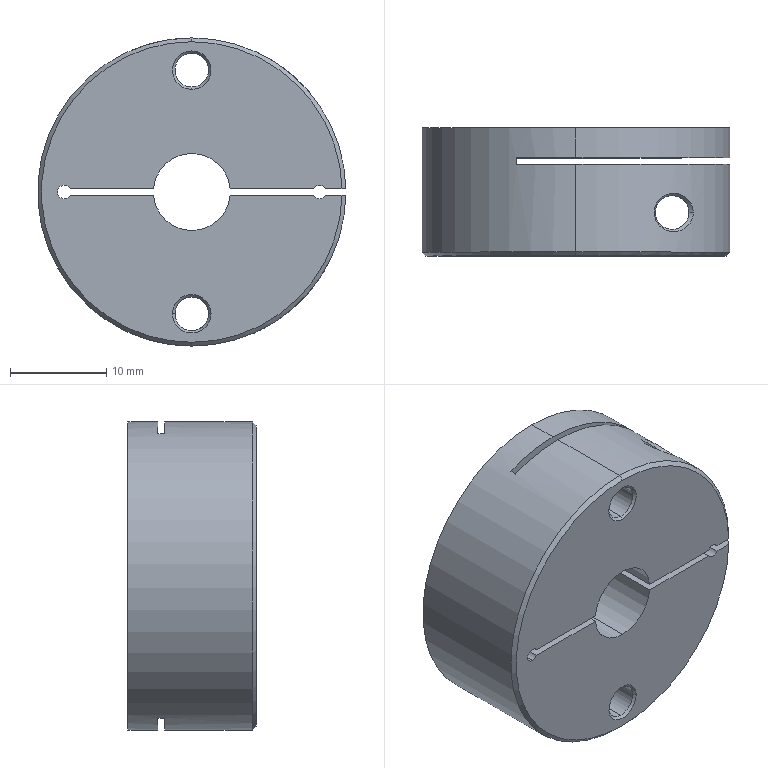Part | NX | 1 solid | 68 faces | box 31.996 x 13.3 x 32 mm | volume 8704 mm3 | cylinder 34 | plane 19 | cone 13 | spline 2 | commonest cylinder face diameters 3.5 x10 1.4 x9 8 x6 32 x5 4.5 x2 7.5 x2